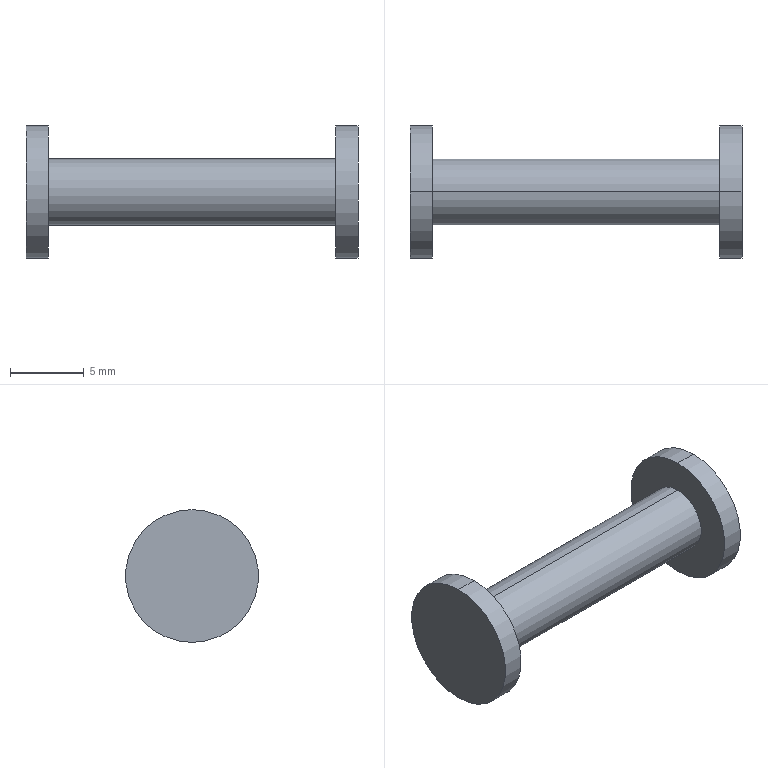Part | SolidWorks | features Revolution 1, Scale 1 | 1 solid | 10 faces | box 22.5 x 9 x 9 mm | volume 500.986 mm3 | cylinder 6 | plane 4 | commonest cylinder face diameters 9 x4 4.5 x2
STEP:
#1=CARTESIAN_POINT('',(-9.75,0.,4.5));
#2=VERTEX_POINT('',#1);
#3=CARTESIAN_POINT('',(-9.75,0.,-4.5));
#4=VERTEX_POINT('',#3);
#5=CARTESIAN_POINT('',(-9.75,0.,0.));
#6=DIRECTION('',(-1.,0.,0.));
#7=DIRECTION('',(0.,0.,1.));
#8=AXIS2_PLACEMENT_3D('',#5,#6,#7);
#9=CIRCLE('',#8,4.5);
#10=EDGE_CURVE('',#2,#4,#9,.T.);
#11=ORIENTED_EDGE('',*,*,#10,.T.);
#12=CARTESIAN_POINT('',(-11.25,0.,-4.5));
#13=VERTEX_POINT('',#12);
#14=CARTESIAN_POINT('',(-11.25,0.,-4.5));
#15=DIRECTION('',(-1.,0.,0.));
#16=VECTOR('',#15,1000.);
#17=LINE('',#14,#16);
#18=EDGE_CURVE('',#4,#13,#17,.T.);
#19=ORIENTED_EDGE('',*,*,#18,.T.);
#20=CARTESIAN_POINT('',(-11.25,0.,4.5));
#21=VERTEX_POINT('',#20);
#22=CARTESIAN_POINT('',(-11.25,0.,0.));
#23=DIRECTION('',(-1.,0.,0.));
#24=DIRECTION('',(0.,0.,1.));
#25=AXIS2_PLACEMENT_3D('',#22,#23,#24);
#26=CIRCLE('',#25,4.5);
#27=EDGE_CURVE('',#21,#13,#26,.T.);
#28=ORIENTED_EDGE('',*,*,#27,.F.);
#29=CARTESIAN_POINT('',(-11.25,0.,4.5));
#30=DIRECTION('',(-1.,0.,0.));
#31=VECTOR('',#30,1000.);
#32=LINE('',#29,#31);
#33=EDGE_CURVE('',#2,#21,#32,.T.);
#34=ORIENTED_EDGE('',*,*,#33,.F.);
#35=EDGE_LOOP('',(#11,#19,#28,#34));
#36=FACE_OUTER_BOUND('',#35,.T.);
#37=CARTESIAN_POINT('',(-11.25,0.,0.));
#38=DIRECTION('',(-1.,0.,0.));
#39=DIRECTION('',(0.,0.,1.));
#40=AXIS2_PLACEMENT_3D('',#37,#38,#39);
#41=CYLINDRICAL_SURFACE('',#40,4.5);
#42=ADVANCED_FACE('',(#36),#41,.T.);
#43=CARTESIAN_POINT('',(9.75,0.,2.25));
#44=VERTEX_POINT('',#43);
#45=CARTESIAN_POINT('',(9.75,0.,-2.25));
#46=VERTEX_POINT('',#45);
#47=CARTESIAN_POINT('',(9.75,0.,0.));
#48=DIRECTION('',(-1.,0.,0.));
#49=DIRECTION('',(0.,0.,1.));
#50=AXIS2_PLACEMENT_3D('',#47,#48,#49);
#51=CIRCLE('',#50,2.25);
#52=EDGE_CURVE('',#44,#46,#51,.T.);
#53=ORIENTED_EDGE('',*,*,#52,.T.);
#54=CARTESIAN_POINT('',(-9.75,0.,-2.25));
#55=VERTEX_POINT('',#54);
#56=CARTESIAN_POINT('',(-11.25,0.,-2.25));
#57=DIRECTION('',(-1.,0.,0.));
#58=VECTOR('',#57,1000.);
#59=LINE('',#56,#58);
#60=EDGE_CURVE('',#46,#55,#59,.T.);
#61=ORIENTED_EDGE('',*,*,#60,.T.);
#62=CARTESIAN_POINT('',(-9.75,0.,2.25));
#63=VERTEX_POINT('',#62);
#64=CARTESIAN_POINT('',(-9.75,0.,0.));
#65=DIRECTION('',(-1.,0.,0.));
#66=DIRECTION('',(0.,0.,1.));
#67=AXIS2_PLACEMENT_3D('',#64,#65,#66);
#68=CIRCLE('',#67,2.25);
#69=EDGE_CURVE('',#63,#55,#68,.T.);
#70=ORIENTED_EDGE('',*,*,#69,.F.);
#71=CARTESIAN_POINT('',(-11.25,0.,2.25));
#72=DIRECTION('',(-1.,0.,0.));
#73=VECTOR('',#72,1000.);
#74=LINE('',#71,#73);
#75=EDGE_CURVE('',#44,#63,#74,.T.);
#76=ORIENTED_EDGE('',*,*,#75,.F.);
#77=EDGE_LOOP('',(#53,#61,#70,#76));
#78=FACE_OUTER_BOUND('',#77,.T.);
#79=CARTESIAN_POINT('',(-11.25,0.,0.));
#80=DIRECTION('',(-1.,0.,0.));
#81=DIRECTION('',(0.,0.,1.));
#82=AXIS2_PLACEMENT_3D('',#79,#80,#81);
#83=CYLINDRICAL_SURFACE('',#82,2.25);
#84=ADVANCED_FACE('',(#78),#83,.T.);
#85=CARTESIAN_POINT('',(11.25,0.,4.5));
#86=VERTEX_POINT('',#85);
#87=CARTESIAN_POINT('',(11.25,0.,-4.5));
#88=VERTEX_POINT('',#87);
#89=CARTESIAN_POINT('',(11.25,0.,0.));
#90=DIRECTION('',(-1.,0.,0.));
#91=DIRECTION('',(0.,0.,1.));
#92=AXIS2_PLACEMENT_3D('',#89,#90,#91);
#93=CIRCLE('',#92,4.5);
#94=EDGE_CURVE('',#86,#88,#93,.T.);
#95=ORIENTED_EDGE('',*,*,#94,.T.);
#96=CARTESIAN_POINT('',(9.75,0.,-4.5));
#97=VERTEX_POINT('',#96);
#98=CARTESIAN_POINT('',(-11.25,0.,-4.5));
#99=DIRECTION('',(-1.,0.,0.));
#100=VECTOR('',#99,1000.);
#101=LINE('',#98,#100);
#102=EDGE_CURVE('',#88,#97,#101,.T.);
#103=ORIENTED_EDGE('',*,*,#102,.T.);
#104=CARTESIAN_POINT('',(9.75,0.,4.5));
#105=VERTEX_POINT('',#104);
#106=CARTESIAN_POINT('',(9.75,0.,0.));
#107=DIRECTION('',(-1.,0.,0.));
#108=DIRECTION('',(0.,0.,1.));
#109=AXIS2_PLACEMENT_3D('',#106,#107,#108);
#110=CIRCLE('',#109,4.5);
#111=EDGE_CURVE('',#105,#97,#110,.T.);
#112=ORIENTED_EDGE('',*,*,#111,.F.);
#113=CARTESIAN_POINT('',(-11.25,0.,4.5));
#114=DIRECTION('',(-1.,0.,0.));
#115=VECTOR('',#114,1000.);
#116=LINE('',#113,#115);
#117=EDGE_CURVE('',#86,#105,#116,.T.);
#118=ORIENTED_EDGE('',*,*,#117,.F.);
#119=EDGE_LOOP('',(#95,#103,#112,#118));
#120=FACE_OUTER_BOUND('',#119,.T.);
#121=CARTESIAN_POINT('',(-11.25,0.,0.));
#122=DIRECTION('',(-1.,0.,0.));
#123=DIRECTION('',(0.,0.,1.));
#124=AXIS2_PLACEMENT_3D('',#121,#122,#123);
#125=CYLINDRICAL_SURFACE('',#124,4.5);
#126=ADVANCED_FACE('',(#120),#125,.T.);
#127=ORIENTED_EDGE('',*,*,#27,.T.);
#128=CARTESIAN_POINT('',(-11.25,0.,0.));
#129=DIRECTION('',(-1.,0.,0.));
#130=DIRECTION('',(0.,0.,1.));
#131=AXIS2_PLACEMENT_3D('',#128,#129,#130);
#132=CIRCLE('',#131,4.5);
#133=EDGE_CURVE('',#13,#21,#132,.T.);
#134=ORIENTED_EDGE('',*,*,#133,.T.);
#135=EDGE_LOOP('',(#127,#134));
#136=FACE_OUTER_BOUND('',#135,.T.);
#137=CARTESIAN_POINT('',(-11.25,4.5,0.));
#138=DIRECTION('',(1.,0.,0.));
#139=DIRECTION('',(0.,0.,-1.));
#140=AXIS2_PLACEMENT_3D('',#137,#138,#139);
#141=PLANE('',#140);
#142=ADVANCED_FACE('',(#136),#141,.F.);
#143=ORIENTED_EDGE('',*,*,#94,.F.);
#144=CARTESIAN_POINT('',(11.25,0.,0.));
#145=DIRECTION('',(-1.,0.,0.));
#146=DIRECTION('',(0.,0.,1.));
#147=AXIS2_PLACEMENT_3D('',#144,#145,#146);
#148=CIRCLE('',#147,4.5);
#149=EDGE_CURVE('',#88,#86,#148,.T.);
#150=ORIENTED_EDGE('',*,*,#149,.F.);
#151=EDGE_LOOP('',(#143,#150));
#152=FACE_OUTER_BOUND('',#151,.T.);
#153=CARTESIAN_POINT('',(11.25,0.,0.));
#154=DIRECTION('',(-1.,0.,0.));
#155=DIRECTION('',(0.,0.,1.));
#156=AXIS2_PLACEMENT_3D('',#153,#154,#155);
#157=PLANE('',#156);
#158=ADVANCED_FACE('',(#152),#157,.F.);
#159=ORIENTED_EDGE('',*,*,#102,.F.);
#160=ORIENTED_EDGE('',*,*,#149,.T.);
#161=ORIENTED_EDGE('',*,*,#117,.T.);
#162=CARTESIAN_POINT('',(9.75,0.,0.));
#163=DIRECTION('',(-1.,0.,0.));
#164=DIRECTION('',(0.,0.,1.));
#165=AXIS2_PLACEMENT_3D('',#162,#163,#164);
#166=CIRCLE('',#165,4.5);
#167=EDGE_CURVE('',#97,#105,#166,.T.);
#168=ORIENTED_EDGE('',*,*,#167,.F.);
#169=EDGE_LOOP('',(#159,#160,#161,#168));
#170=FACE_OUTER_BOUND('',#169,.T.);
#171=CARTESIAN_POINT('',(-11.25,0.,0.));
#172=DIRECTION('',(-1.,0.,0.));
#173=DIRECTION('',(0.,0.,1.));
#174=AXIS2_PLACEMENT_3D('',#171,#172,#173);
#175=CYLINDRICAL_SURFACE('',#174,4.5);
#176=ADVANCED_FACE('',(#170),#175,.T.);
#177=ORIENTED_EDGE('',*,*,#52,.F.);
#178=CARTESIAN_POINT('',(9.75,0.,0.));
#179=DIRECTION('',(-1.,0.,0.));
#180=DIRECTION('',(0.,0.,1.));
#181=AXIS2_PLACEMENT_3D('',#178,#179,#180);
#182=CIRCLE('',#181,2.25);
#183=EDGE_CURVE('',#46,#44,#182,.T.);
#184=ORIENTED_EDGE('',*,*,#183,.F.);
#185=EDGE_LOOP('',(#177,#184));
#186=FACE_BOUND('',#185,.T.);
#187=ORIENTED_EDGE('',*,*,#111,.T.);
#188=ORIENTED_EDGE('',*,*,#167,.T.);
#189=EDGE_LOOP('',(#187,#188));
#190=FACE_OUTER_BOUND('',#189,.T.);
#191=CARTESIAN_POINT('',(9.75,4.5,0.));
#192=DIRECTION('',(1.,0.,0.));
#193=DIRECTION('',(0.,0.,-1.));
#194=AXIS2_PLACEMENT_3D('',#191,#192,#193);
#195=PLANE('',#194);
#196=ADVANCED_FACE('',(#186,#190),#195,.F.);
#197=ORIENTED_EDGE('',*,*,#60,.F.);
#198=ORIENTED_EDGE('',*,*,#183,.T.);
#199=ORIENTED_EDGE('',*,*,#75,.T.);
#200=CARTESIAN_POINT('',(-9.75,0.,0.));
#201=DIRECTION('',(-1.,0.,0.));
#202=DIRECTION('',(0.,0.,1.));
#203=AXIS2_PLACEMENT_3D('',#200,#201,#202);
#204=CIRCLE('',#203,2.25);
#205=EDGE_CURVE('',#55,#63,#204,.T.);
#206=ORIENTED_EDGE('',*,*,#205,.F.);
#207=EDGE_LOOP('',(#197,#198,#199,#206));
#208=FACE_OUTER_BOUND('',#207,.T.);
#209=CARTESIAN_POINT('',(-11.25,0.,0.));
#210=DIRECTION('',(-1.,0.,0.));
#211=DIRECTION('',(0.,0.,1.));
#212=AXIS2_PLACEMENT_3D('',#209,#210,#211);
#213=CYLINDRICAL_SURFACE('',#212,2.25);
#214=ADVANCED_FACE('',(#208),#213,.T.);
#215=ORIENTED_EDGE('',*,*,#10,.F.);
#216=CARTESIAN_POINT('',(-9.75,0.,0.));
#217=DIRECTION('',(-1.,0.,0.));
#218=DIRECTION('',(0.,0.,1.));
#219=AXIS2_PLACEMENT_3D('',#216,#217,#218);
#220=CIRCLE('',#219,4.5);
#221=EDGE_CURVE('',#4,#2,#220,.T.);
#222=ORIENTED_EDGE('',*,*,#221,.F.);
#223=EDGE_LOOP('',(#215,#222));
#224=FACE_OUTER_BOUND('',#223,.T.);
#225=ORIENTED_EDGE('',*,*,#69,.T.);
#226=ORIENTED_EDGE('',*,*,#205,.T.);
#227=EDGE_LOOP('',(#225,#226));
#228=FACE_BOUND('',#227,.T.);
#229=CARTESIAN_POINT('',(-9.75,2.25,0.));
#230=DIRECTION('',(-1.,0.,0.));
#231=DIRECTION('',(0.,0.,1.));
#232=AXIS2_PLACEMENT_3D('',#229,#230,#231);
#233=PLANE('',#232);
#234=ADVANCED_FACE('',(#224,#228),#233,.F.);
#235=ORIENTED_EDGE('',*,*,#18,.F.);
#236=ORIENTED_EDGE('',*,*,#221,.T.);
#237=ORIENTED_EDGE('',*,*,#33,.T.);
#238=ORIENTED_EDGE('',*,*,#133,.F.);
#239=EDGE_LOOP('',(#235,#236,#237,#238));
#240=FACE_OUTER_BOUND('',#239,.T.);
#241=CARTESIAN_POINT('',(-11.25,0.,0.));
#242=DIRECTION('',(-1.,0.,0.));
#243=DIRECTION('',(0.,0.,1.));
#244=AXIS2_PLACEMENT_3D('',#241,#242,#243);
#245=CYLINDRICAL_SURFACE('',#244,4.5);
#246=ADVANCED_FACE('',(#240),#245,.T.);
#247=CLOSED_SHELL('',(#42,#84,#126,#142,#158,#176,#196,#214,#234,#246));
#248=MANIFOLD_SOLID_BREP('',#247);
#249=CARTESIAN_POINT('',(0.,0.,0.));
#250=DIRECTION('',(0.,0.,1.));
#251=DIRECTION('',(1.,0.,0.));
#252=AXIS2_PLACEMENT_3D('',#249,#250,#251);
#253=(LENGTH_UNIT()NAMED_UNIT(*)SI_UNIT(.MILLI.,.METRE.));
#254=UNCERTAINTY_MEASURE_WITH_UNIT(LENGTH_MEASURE(0.00001),#253,'','');
#255=(NAMED_UNIT(*)PLANE_ANGLE_UNIT()SI_UNIT($,.RADIAN.));
#256=(NAMED_UNIT(*)SI_UNIT($,.STERADIAN.)SOLID_ANGLE_UNIT());
#257=(GEOMETRIC_REPRESENTATION_CONTEXT(3)GLOBAL_UNCERTAINTY_ASSIGNED_CONTEXT((#254))GLOBAL_UNIT_ASSIGNED_CONTEXT((#253,#255,#256))REPRESENTATION_CONTEXT('',''));
#258=ADVANCED_BREP_SHAPE_REPRESENTATION('',(#248,#252),#257);